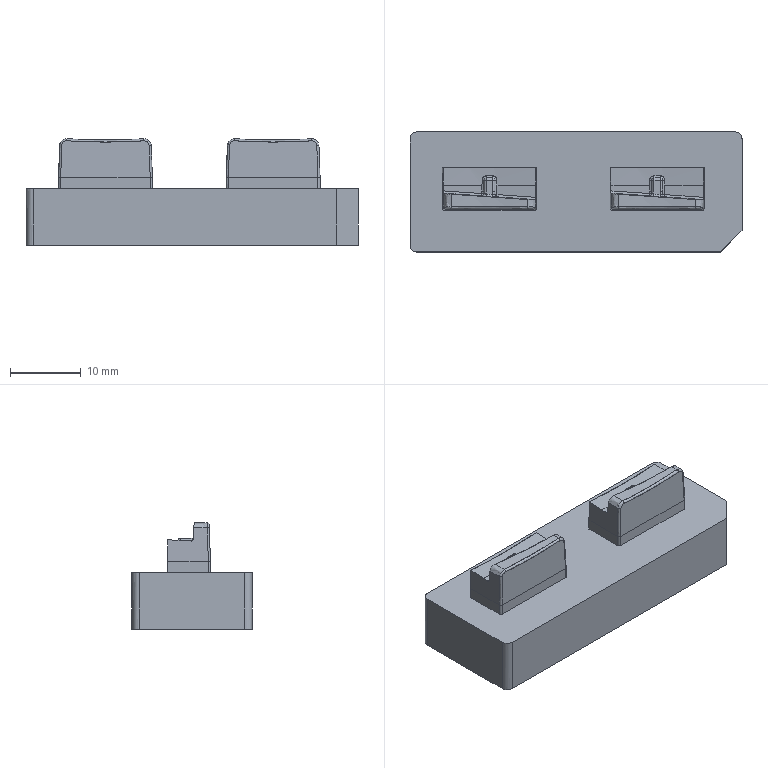NC program | PowerMill | posted with a generic post | part box 47 x 17 x 15.061 mm
Lines 1 to 1048 of 212044:
%
O0001
N104 ( POWERMILL CB  : 2026004.0)
N105 ( POST VER      : 2026.0.0.5161)
N106 ( OPTION FILE   : FANUC)
N107 ( OUTPUT WORKPLANE : WORLD)
N108 (  )
N109 ( TOOL LIST )
N110 (---------------------------------------)
N111 ( NO. | ID        | DIA.| TIP RAD|LENGTH)
N112 (---------------------------------------)
N113 (    1|D10C_1_1   |10.0 |  0.0   |70.52 )
N114 (    2|D4C_1_1    | 4.0 |  0.0   |62.24 )
N115 (   27|D1C_1_1    | 1.0 |  0.0   |58.04 )
N116 (    3|D10_1_1    |10.0 |  0.0   |70.24 )
N117 (    4|R1_1_1     | 2.0 |  1.0   |61.84 )
N118 (    6|R0.5_1_1   | 1.0 |  0.5   |58.16 )
N119 (   25|R0.3_1_1   | 0.6 |  0.3   |58.08 )
N120 (   13|TEXT_D4_1_1| 4.0 |  0.3   |62.32 )
N121 (---------------------------------------)
N122 (  )
N123 ( NUMBER OF TOOLPATHS: 13.0 )
N124 ( ESTIMATED PROGRAM DURATION: 0 HOURS 20 MIN 46 SEC)
N125 (  )
N126 G00 G21 G80 G40 G17
N127 G90
N128 G54
N129 G53 Z0.0
N130 (---------------)
N131 ( START TOOLPATH : 精公开粗01-扫面平行-D10C )
N132 (---------------)
N133 ( TOOL NO.    :1 )
N134 ( TOOL TYPE   : ENDMILL)
N135 ( TOOL ID     : D10C_1_1)
N136 ( TOOL DIA    : 10.0 LENGTH 70.52)
N137 T1
N138 M6
N139 S8000 M03
N140 G00 G90 X0.0 Y0.0
N141 G43 Z10.2 H1
N142
N143 G05 P10000 R4
N144 X31.28 Y11.28
N145 Z1.131
N146 G01 Z-0.069 F6000.0
N147 X26.28 F10000.0
N148 X-26.28
N149 Y5.64
N150 X26.28
N151 Y0.0
N152 X-26.28
N153 Y-5.64
N154 X26.28
N155 Y-11.28
N156 X-26.28
N157 X-31.28
N158 G00 Z10.2
N159 G05 P0
N160 (---------------)
N161 ( END TOOLPATH : 精公开粗01-扫面平行-D10C )
N162 (---------------)
N163 ( START TOOLPATH : 精公开粗01-外形偏置-D10C )
N164 (---------------)
N165 G00 X-0.2 Y0.0 Z9.881
N166 G05 P10000 R4
N167 X31.555 Y4.0124
N168 Z0.7186
N169 G01 Z-0.4814 F6000.0
N170 X31.0275 F10000.0
N171 G03 X26.28 Y-0.7351 I0.0 J-4.7475
N172 G01 Y-10.28
N173 G02 X25.28 Y-11.28 I-1.0 J0.0
N174 G01 X-25.68
N175 G02 X-26.68 Y-10.28 I0.0 J1.0
N176 G01 Y10.28
N177 G02 X-25.68 Y11.28 I1.0 J0.0
N178 G01 X25.28
N179 G02 X26.28 Y10.28 I0.0 J-1.0
N180 G01 Y-0.7351
N181 X22.9506 Y-0.9668
N182 X22.9641 Y-1.1601
N183 X22.933 Y-2.707
N184 X22.7913 Y-3.4804
N185 X22.5391 Y-4.2538
N186 X22.1429 Y-5.0273
N187 X21.5582 Y-5.8007
N188 X20.7183 Y-6.5741
N189 X19.9091 Y-7.0696
N190 X19.2573 Y-7.3476
N191 X18.3622 Y-7.5959
N192 X17.5888 Y-7.6917
N193 X16.8154 Y-7.7121
N194 X11.4014 Y-7.6611
N195 X11.3967
N196 X5.9874 Y-7.7126
N197 X5.214 Y-7.6816
N198 X4.4406 Y-7.5712
N199 X3.6738 Y-7.3476
N200 X2.8937 Y-7.0001
N201 X2.223 Y-6.5741
N202 X1.3803 Y-5.8007
N203 X0.7978 Y-5.0273
N204 X0.5734 Y-4.6294
N205 X0.4007 Y-4.2538
N206 X0.1489 Y-3.4804
N207 X0.0079 Y-2.707
N208 X-0.0194 Y-1.9336
N209 X-0.0237 Y-1.1757
N210 X-0.7788 Y-1.1601
N211 X-0.8107 Y-2.707
N212 X-0.9518 Y-3.4804
N213 X-1.2049 Y-4.2538
N214 X-1.6016 Y-5.0273
N215 X-1.7469 Y-5.2497
N216 X-2.1858 Y-5.8007
N217 X-2.5203 Y-6.1467
N218 X-3.0233 Y-6.5741
N219 X-3.2937 Y-6.7631
N220 X-4.0671 Y-7.1796
N221 X-4.4858 Y-7.3476
N222 X-4.8406 Y-7.4671
N223 X-5.614 Y-7.6365
N224 X-6.3874 Y-7.704
N225 X-11.8014 Y-7.6651
N226 X-11.805
N227 X-17.9888 Y-7.7098
N228 X-18.7622 Y-7.6593
N229 X-19.5357 Y-7.5155
N230 X-20.3091 Y-7.2523
N231 X-21.0825 Y-6.8685
N232 X-21.5226 Y-6.5741
N233 X-21.8559 Y-6.3049
N234 X-22.364 Y-5.8007
N235 X-22.6294 Y-5.4834
N236 X-22.9463 Y-5.0273
N237 X-23.3432 Y-4.2538
N238 X-23.594 Y-3.4804
N239 X-23.7368 Y-2.707
N240 X-23.7641 Y-1.9336
N241 X-23.7721 Y-0.3867
N242 X-23.73 Y0.3867
N243 X-23.573 Y1.1601
N244 X-23.4028 Y1.6681
N245 X-23.2893 Y1.9336
N246 X-22.8515 Y2.707
N247 X-22.6294 Y3.006
N248 X-22.2028 Y3.4804
N249 X-21.8559 Y3.795
N250 X-21.2044 Y4.2538
N251 X-20.3091 Y4.6806
N252 X-19.5357 Y4.8996
N253 X-18.7622 Y4.9981
N254 X-17.9888 Y4.9861
N255 X-5.614 Y4.1201
N256 X-4.8406 Y3.9942
N257 X-4.0671 Y3.7451
N258 X-3.2937 Y3.3525
N259 X-2.5203 Y2.773
N260 X-1.769 Y1.9336
N261 X-1.3083 Y1.1601
N262 X-1.005 Y0.3867
N263 X-0.8337 Y-0.3867
N264 X-0.7788 Y-1.1601
N265 X-0.0237 Y-1.1757
N266 X-0.0283 Y-0.3867
N267 X0.0143 Y0.3867
N268 X0.1704 Y1.1601
N269 X0.4548 Y1.9336
N270 X0.5734 Y2.177
N271 X0.8933 Y2.707
N272 X1.3469 Y3.2768
N273 X1.5396 Y3.4804
N274 X2.1203 Y3.9724
N275 X2.5408 Y4.2538
N276 X2.8937 Y4.4455
N277 X3.6671 Y4.7591
N278 X4.4406 Y4.9414
N279 X5.214 Y5.0062
N280 X5.9874 Y4.9703
N281 X17.5888 Y4.1592
N282 X18.3622 Y4.0955
N283 X19.1357 Y3.9326
N284 X19.9091 Y3.6434
N285 X20.2305 Y3.4804
N286 X20.6825 Y3.2017
N287 X21.2965 Y2.707
N288 X21.4559 Y2.5509
N289 X21.9755 Y1.9336
N290 X22.2294 Y1.5464
N291 X22.436 Y1.1601
N292 X22.7398 Y0.3867
N293 X22.9102 Y-0.3867
N294 X22.9506 Y-0.9668
N295 X26.28 Y-0.7351
N296 G00 Z3.3563
N297 G01 X31.555 Y4.0124
N298 G00 Z0.3563
N299 G01 Z-0.8437 F6000.0
N300 X31.0275 F10000.0
N301 G03 X26.28 Y-0.7351 I0.0 J-4.7475
N302 G01 Y-10.28
N303 G02 X25.28 Y-11.28 I-1.0 J0.0
N304 G01 X-25.68
N305 G02 X-26.68 Y-10.28 I0.0 J1.0
N306 G01 Y10.28
N307 G02 X-25.68 Y11.28 I1.0 J0.0
N308 G01 X25.28
N309 G02 X26.28 Y10.28 I0.0 J-1.0
N310 G01 Y-0.6564
N311 X23.1598 Y-0.8701
N312 X23.1797 Y-1.1601
N313 X23.1499 Y-2.707
N314 X23.0133 Y-3.4804
N315 X22.7652 Y-4.2538
N316 X22.3726 Y-5.0273
N317 X21.8112 Y-5.8007
N318 X21.4559 Y-6.1752
N319 X20.9868 Y-6.5741
N320 X20.6825 Y-6.7872
N321 X19.9091 Y-7.2199
N322 X19.6073 Y-7.3476
N323 X19.1357 Y-7.5058
N324 X18.3622 Y-7.6665
N325 X17.5888 Y-7.7263
N326 X5.214 Y-7.7236
N327 X4.4406 Y-7.6464
N328 X3.6671 Y-7.4647
N329 X3.33 Y-7.3476
N330 X2.8937 Y-7.1538
N331 X2.1203 Y-6.6982
N332 X1.9499 Y-6.5741
N333 X1.3469 Y-6.0418
N334 X1.1262 Y-5.8007
N335 X0.5734 Y-5.0459
N336 X0.1714 Y-4.2538
N337 X-0.0785 Y-3.4804
N338 X-0.2 Y-2.8258
N339 X-0.2395 Y-1.9336
N340 X-0.2407 Y-1.1666
N341 X-0.5638 Y-1.1601
N342 X-0.5945 Y-2.707
N343 X-0.7306 Y-3.4804
N344 X-0.9734 Y-4.2399
N345 X-1.3713 Y-5.0273
N346 X-1.7469 Y-5.5717
N347 X-1.9327 Y-5.8007
N348 X-2.5203 Y-6.3844
N349 X-2.7572 Y-6.5741
N350 X-3.2937 Y-6.9312
N351 X-4.1359 Y-7.3476
N352 X-4.8406 Y-7.5644
N353 X-5.614 Y-7.6964
N354 X-6.3874 Y-7.7263
N355 X-17.9888
N356 X-18.7622 Y-7.712
N357 X-19.5357 Y-7.6034
N358 X-20.3091 Y-7.3868
N359 X-21.0825 Y-7.0321
N360 X-21.7943 Y-6.5741
N361 X-22.6177 Y-5.8007
N362 X-23.1815 Y-5.0273
N363 X-23.4028 Y-4.6283
N364 X-23.5726 Y-4.2538
N365 X-23.8216 Y-3.4804
N366 X-23.9579 Y-2.707
N367 X-23.9838 Y-1.9336
N368 X-23.9863 Y-0.3867
N369 X-23.9489 Y0.3867
N370 X-23.7967 Y1.1601
N371 X-23.5169 Y1.9336
N372 X-23.085 Y2.707
N373 X-22.6294 Y3.2897
N374 X-22.4489 Y3.4804
N375 X-21.8559 Y3.9933
N376 X-21.4711 Y4.2538
N377 X-21.0825 Y4.4704
N378 X-20.3091 Y4.7847
N379 X-19.5357 Y4.9702
N380 X-19.0108 Y5.0273
N381 X-18.3916
N382 X-5.614 Y4.1345
N383 X-4.8406 Y4.0403
N384 X-4.0671 Y3.8286
N385 X-3.2937 Y3.4779
N386 X-2.5203 Y2.9594
N387 X-2.2308 Y2.707
N388 X-1.7469 Y2.1869
N389 X-1.5526 Y1.9336
N390 X-1.0916 Y1.1601
N391 X-0.7898 Y0.3867
N392 X-0.6172 Y-0.3867
N393 X-0.5638 Y-1.1601
N394 X-0.2407 Y-1.1666
N395 X-0.2419 Y-0.3867
N396 X-0.2049 Y0.3867
N397 X-0.0528 Y1.1601
N398 X0.227 Y1.9336
N399 X0.6588 Y2.707
N400 X1.295 Y3.4804
N401 X2.1203 Y4.1564
N402 X2.8937 Y4.5806
N403 X3.6671 Y4.8532
N404 X4.4406 Y5.0002
N405 X4.733 Y5.0273
N406 X5.3521
N407 X18.3622 Y4.117
N408 X19.1357 Y3.9899
N409 X19.9091 Y3.7381
N410 X20.4493 Y3.4804
N411 X20.6825 Y3.3428
N412 X21.4559 Y2.7598
N413 X22.1912 Y1.9336
N414 X22.6517 Y1.1601
N415 X22.9538 Y0.3867
N416 X23.1267 Y-0.3867
N417 X23.1598 Y-0.8701
N418 X26.28 Y-0.6564
N419 Y-0.7351
N420 G00 Z2.9939
N421 G01 X31.555 Y4.0124
N422 G00 Z-0.0061
N423 G01 Z-1.2061 F6000.0
N424 X31.0275 F10000.0
N425 G03 X26.28 Y-0.7351 I0.0 J-4.7475
N426 G01 Y-10.28
N427 G02 X25.28 Y-11.28 I-1.0 J0.0
N428 G01 X-25.68
N429 G02 X-26.68 Y-10.28 I0.0 J1.0
N430 G01 Y10.28
N431 G02 X-25.68 Y11.28 I1.0 J0.0
N432 G01 X25.28
N433 G02 X26.28 Y10.28 I0.0 J-1.0
N434 G01 Y-0.6635
N435 X23.2292 Y-0.8701
N436 X23.2489 Y-1.1601
N437 X23.2498 Y-1.9336
N438 X23.22 Y-2.707
N439 X23.0864 Y-3.4804
N440 X23.0028 Y-3.7922
N441 X22.8382 Y-4.2538
N442 X22.4558 Y-5.0273
N443 X22.2294 Y-5.3724
N444 X21.8943 Y-5.8007
N445 X21.4559 Y-6.2554
N446 X21.0766 Y-6.5741
N447 X20.6825 Y-6.8542
N448 X19.7198 Y-7.3476
N449 X19.1357 Y-7.5362
N450 X18.3622 Y-7.6927
N451 X17.5888 Y-7.7389
N452 X5.214 Y-7.7377
N453 X4.4406 Y-7.6676
N454 X3.6671 Y-7.4911
N455 X3.2539 Y-7.3476
N456 X2.8937 Y-7.1899
N457 X2.1203 Y-6.7382
N458 X1.8988 Y-6.5741
N459 X1.3469 Y-6.0901
N460 X1.0801 Y-5.8007
N461 X0.5734 Y-5.1141
N462 X0.1353 Y-4.2538
N463 X-0.1106 Y-3.4804
N464 X-0.2456 Y-2.707
N465 X-0.2739 Y-1.9336
N466 X-0.275 Y-1.1598
N467 X-0.4953 Y-1.1601
N468 X-0.4941 Y-1.9336
N469 X-0.5239 Y-2.707
N470 X-0.6575 Y-3.4804
N471 X-0.9062 Y-4.2538
N472 X-1.2902 Y-5.0273
N473 X-1.7469 Y-5.6768
N474 X-2.5203 Y-6.4571
N475 X-3.2937 Y-6.9965
N476 X-4.0257 Y-7.3476
N477 X-4.8406 Y-7.5957
N478 X-5.614 Y-7.7181
N479 X-6.3874 Y-7.739
N480 X-17.9888
N481 X-18.7622 Y-7.729
N482 X-19.5357 Y-7.6238
N483 X-20.3091 Y-7.4152
N484 X-21.0825 Y-7.0723
N485 X-21.8449 Y-6.5741
N486 X-22.6294 Y-5.8404
N487 X-23.2239 Y-5.0273
N488 X-23.4028 Y-4.7049
N489 X-23.6082 Y-4.2538
N490 X-23.8545 Y-3.4804
N491 X-23.9895 Y-2.707
N492 X-24.0181 Y-1.9336
N493 X-24.0202 Y-0.3867
N494 X-23.9845 Y0.3867
N495 X-23.8346 Y1.1601
N496 X-23.5576 Y1.9336
N497 X-23.4028 Y2.2496
N498 X-23.1294 Y2.707
N499 X-22.4987 Y3.4804
N500 X-21.8559 Y4.0347
N501 X-21.5315 Y4.2538
N502 X-21.0825 Y4.504
N503 X-20.3091 Y4.8136
N504 X-19.5357 Y4.9916
N505 X-18.7622 Y5.052
N506 X-18.2055 Y5.0273
N507 X-5.614 Y4.1468
N508 X-4.8406 Y4.061
N509 X-4.0671 Y3.8601
N510 X-3.2937 Y3.5252
N511 X-2.5203 Y3.0238
N512 X-2.1524 Y2.707
N513 X-1.7469 Y2.2795
N514 X-1.4777 Y1.9336
N515 X-1.0196 Y1.1601
N516 X-0.7189 Y0.3867
N517 X-0.5475 Y-0.3867
N518 X-0.4953 Y-1.1601
N519 X-0.275 Y-1.1598
N520 X-0.2761 Y-0.3867
N521 X-0.2406 Y0.3867
N522 X-0.0907 Y1.1601
N523 X0.1863 Y1.9336
N524 X0.5734 Y2.6446
N525 X1.2452 Y3.4804
N526 X2.1203 Y4.1951
N527 X2.8937 Y4.612
N528 X3.6671 Y4.8799
N529 X4.4406 Y5.0217
N530 X5.214 Y5.0476
N531 X18.3622 Y4.1306
N532 X19.1357 Y4.0139
N533 X19.9091 Y3.775
N534 X20.5348 Y3.4804
N535 X21.4559 Y2.8316
N536 X21.5916 Y2.707
N537 X22.2294 Y1.9853
N538 X22.7243 Y1.1601
N539 X23.0028 Y0.4646
N540 X23.1965 Y-0.3867
N541 X23.2292 Y-0.8701
N542 X26.28 Y-0.6635
N543 Y-0.7351
N544 G00 Z2.6316
N545 G01 X31.555 Y4.0124
N546 G00 Z-0.3684
N547 G01 Z-1.5684 F6000.0
N548 X31.0275 F10000.0
N549 G03 X26.28 Y-0.7351 I0.0 J-4.7475
N550 G01 Y-10.28
N551 G02 X25.28 Y-11.28 I-1.0 J0.0
N552 G01 X-25.68
N553 G02 X-26.68 Y-10.28 I0.0 J1.0
N554 G01 Y10.28
N555 G02 X-25.68 Y11.28 I1.0 J0.0
N556 G01 X25.28
N557 G02 X26.28 Y10.28 I0.0 J-1.0
N558 G01 Y-0.6677
N559 X23.2442 Y-0.8701
N560 X23.2636 Y-1.1601
N561 X23.2497 Y-1.906
N562 X23.2498 Y-1.9336
N563 X23.2487 Y-1.9607
N564 X23.2349 Y-2.707
N565 X23.0975 Y-3.4804
N566 X23.0181 Y-3.7348
N567 X23.0027 Y-3.7922
N568 X22.9828 Y-3.8482
N569 X22.8562 Y-4.2538
N570 X22.4758 Y-5.0273
N571 X22.2294 Y-5.4027
N572 X21.9126 Y-5.8007
N573 X21.4559 Y-6.2702
N574 X21.1046 Y-6.5741
N575 X20.6825 Y-6.8757
N576 X19.7593 Y-7.3476
N577 X19.1357 Y-7.5492
N578 X18.3622 Y-7.7072
N579 X17.5888 Y-7.7516
N580 X5.214 Y-7.7508
N581 X4.4406 Y-7.6821
N582 X3.6671 Y-7.5068
N583 X3.2105 Y-7.3476
N584 X2.8937 Y-7.2084
N585 X2.1203 Y-6.7594
N586 X1.8704 Y-6.5741
N587 X1.3469 Y-6.1142
N588 X1.0572 Y-5.8007
N589 X0.5734 Y-5.1464
N590 X0.118 Y-4.2538
N591 X-0.1259 Y-3.4804
N592 X-0.2595 Y-2.707
N593 X-0.2868 Y-1.9336
N594 X-0.2879 Y-1.1637
N595 X-0.4804 Y-1.1601
N596 X-0.4942 Y-1.9081
N597 Y-1.9336
N598 X-0.4952 Y-1.9592
N599 X-0.509 Y-2.707
N600 X-0.6465 Y-3.4804
N601 X-0.8878 Y-4.2538
N602 X-1.2681 Y-5.0273
N603 X-1.7469 Y-5.7022
N604 X-2.5203 Y-6.4773
N605 X-3.2937 Y-7.0165
N606 X-3.9846 Y-7.3476
N607 X-4.8406 Y-7.6084
N608 X-5.614 Y-7.7317
N609 X-6.3874 Y-7.7516
N610 X-17.9888
N611 X-18.7622 Y-7.7422
N612 X-19.5357 Y-7.6389
N613 X-20.3091 Y-7.4317
N614 X-21.0825 Y-7.0914
N615 X-21.8559 Y-6.5876
N616 X-22.6294 Y-5.8665
N617 X-23.244 Y-5.0273
N618 X-23.4028 Y-4.7419
N619 X-23.6245 Y-4.2538
N620 X-23.8698 Y-3.4804
N621 X-24.0032 Y-2.707
N622 X-24.0307 Y-1.9336
N623 X-24.0329 Y-0.3867
N624 X-23.9988 Y0.3867
N625 X-23.851 Y1.1601
N626 X-23.5763 Y1.9336
N627 X-23.4028 Y2.2866
N628 X-23.1511 Y2.707
N629 X-22.6294 Y3.3704
N630 X-21.8559 Y4.0574
N631 X-21.5657 Y4.2538
N632 X-21.0825 Y4.5239
N633 X-20.3091 Y4.8313
N634 X-19.5357 Y5.0071
N635 X-18.7622 Y5.066
N636 X-17.9888 Y5.0248
N637 X-5.614 Y4.1595
N638 X-4.8406 Y4.0757
N639 X-4.0671 Y3.8767
N640 X-3.2937 Y3.5454
N641 X-2.5203 Y3.0461
N642 X-2.126 Y2.707
N643 X-1.7469 Y2.3076
N644 X-1.4551 Y1.9336
N645 X-0.9995 Y1.1601
N646 X-0.7008 Y0.3867
N647 X-0.5319 Y-0.3867
N648 X-0.4804 Y-1.1601
N649 X-0.2879 Y-1.1637
N650 X-0.289 Y-0.3867
N651 X-0.255 Y0.3867
N652 X-0.107 Y1.1601
N653 X0.1676 Y1.9336
N654 X0.5734 Y2.6776
N655 X1.2193 Y3.4804
N656 X1.3469 Y3.6063
N657 X2.1203 Y4.2169
N658 X2.8937 Y4.631
N659 X3.6671 Y4.8967
N660 X4.3576 Y5.0273
N661 X5.214 Y5.0606
N662 X18.3622 Y4.1432
N663 X19.1357 Y4.0299
N664 X19.9091 Y3.7932
N665 X20.569 Y3.4804
N666 X21.4559 Y2.8547
N667 X21.6179 Y2.707
N668 X22.2294 Y2.0157
N669 X22.7444 Y1.1601
N670 X23.0028 Y0.5146
N671 X23.212 Y-0.3867
N672 X23.2442 Y-0.8701
N673 X26.28 Y-0.6677
N674 Y-0.7351
N675 G00 Z2.2692
N676 G01 X31.555 Y4.0124
N677 G00 Z-0.7308
N678 G01 Z-1.9308 F6000.0
N679 X31.0275 F10000.0
N680 G03 X26.28 Y-0.7351 I0.0 J-4.7475
N681 G01 Y-10.28
N682 G02 X25.28 Y-11.28 I-1.0 J0.0
N683 G01 X-25.68
N684 G02 X-26.68 Y-10.28 I0.0 J1.0
N685 G01 Y10.28
N686 G02 X-25.68 Y11.28 I1.0 J0.0
N687 G01 X25.28
N688 G02 X26.28 Y10.28 I0.0 J-1.0
N689 G01 Y-0.675
N690 X23.2575 Y-0.8701
N691 X23.2762 Y-1.1601
N692 X23.2487 Y-2.707
N693 X23.1133 Y-3.4804
N694 X22.8738 Y-4.2538
N695 X22.4958 Y-5.0273
N696 X22.2294 Y-5.4327
N697 X21.936 Y-5.8007
N698 X21.4559 Y-6.2944
N699 X21.1329 Y-6.5741
N700 X20.6825 Y-6.8962
N701 X19.8034 Y-7.3476
N702 X19.1357 Y-7.5652
N703 X18.3622 Y-7.7216
N704 X17.5888 Y-7.7643
N705 X5.214 Y-7.7639
N706 X4.4406 Y-7.6967
N707 X3.6671 Y-7.5225
N708 X3.1671 Y-7.3476
N709 X2.8937 Y-7.227
N710 X2.1203 Y-6.7806
N711 X1.842 Y-6.5741
N712 X1.3469 Y-6.1377
N713 X1.0343 Y-5.8007
N714 X0.5734 Y-5.1788
N715 X0.1007 Y-4.2538
N716 X-0.1413 Y-3.4804
N717 X-0.2734 Y-2.707
N718 X-0.2994 Y-1.9336
N719 X-0.3005 Y-1.1631
N720 X-0.4677 Y-1.1601
N721 X-0.4952 Y-2.707
N722 X-0.6307 Y-3.4804
N723 X-0.8703 Y-4.2538
N724 X-0.9734 Y-4.4996
N725 X-1.2481 Y-5.0273
N726 X-1.7469 Y-5.7298
N727 X-2.5203 Y-6.5005
N728 X-3.2937 Y-7.0362
N729 X-3.9405 Y-7.3476
N730 X-4.8406 Y-7.6239
N731 X-5.614 Y-7.7454
N732 X-6.3874 Y-7.7643
N733 X-17.9888
N734 X-18.7622 Y-7.7555
N735 X-19.5357 Y-7.654
N736 X-20.3091 Y-7.4482
N737 X-20.5775 Y-7.3476
N738 X-21.0825 Y-7.1106
N739 X-21.8559 Y-6.6098
N740 X-22.6294 Y-5.8926
N741 X-23.264 Y-5.0273
N742 X-23.4028 Y-4.779
N743 X-23.642 Y-4.2538
N744 X-23.8852 Y-3.4804
N745 X-24.017 Y-2.707
N746 X-24.0434 Y-1.9336
N747 X-24.0455 Y-0.3867
N748 X-24.013 Y0.3867
N749 X-23.8673 Y1.1601
N750 X-23.595 Y1.9336
N751 X-23.4028 Y2.3236
N752 X-23.1727 Y2.707
N753 X-22.6294 Y3.3976
N754 X-21.8559 Y4.0802
N755 X-21.5998 Y4.2538
N756 X-21.0825 Y4.5437
N757 X-20.3091 Y4.8491
N758 X-19.5357 Y5.0225
N759 X-18.7622 Y5.08
N760 X-17.9888 Y5.0377
N761 X-5.614 Y4.1722
N762 X-4.8406 Y4.0904
N763 X-4.0671 Y3.8933
N764 X-3.2937 Y3.5643
N765 X-2.5203 Y3.068
N766 X-2.101 Y2.707
N767 X-1.7469 Y2.3342
N768 X-1.4341 Y1.9336
N769 X-0.9812 Y1.1601
N770 X-0.6847 Y0.3867
N771 X-0.5176 Y-0.3867
N772 X-0.4677 Y-1.1601
N773 X-0.3005 Y-1.1631
N774 X-0.3016 Y-0.3867
N775 X-0.2694 Y0.3867
N776 X-0.1234 Y1.1601
N777 X0.1489 Y1.9336
N778 X0.5711 Y2.707
N779 X1.1934 Y3.4804
N780 X1.3469 Y3.6319
N781 X2.1203 Y4.2387
N782 X2.8937 Y4.6501
N783 X3.6671 Y4.9136
N784 X4.2419 Y5.0273
N785 X5.214 Y5.0737
N786 X18.3622 Y4.1559
N787 X19.1357 Y4.0449
N788 X19.9091 Y3.81
N789 X20.6026 Y3.4804
N790 X21.4559 Y2.8778
N791 X21.643 Y2.707
N792 X22.2294 Y2.0447
N793 X22.7627 Y1.1601
N794 X23.0028 Y0.5646
N795 X23.2263 Y-0.3867
N796 X23.2575 Y-0.8701
N797 X26.28 Y-0.675
N798 Y-0.7351
N799 G00 Z1.9069
N800 G01 X31.555 Y4.0124
N801 G00 Z-1.0931
N802 G01 Z-2.2931 F6000.0
N803 X31.0275 F10000.0
N804 G03 X26.28 Y-0.7351 I0.0 J-4.7475
N805 G01 Y-0.7793
N806 X23.2768 Y-0.9668
N807 X23.2889 Y-1.1601
N808 X23.2624 Y-2.707
N809 X23.1291 Y-3.4804
N810 X22.8913 Y-4.2538
N811 X22.5157 Y-5.0273
N812 X22.2294 Y-5.4628
N813 X21.9593 Y-5.8007
N814 X21.4559 Y-6.3186
N815 X21.1611 Y-6.5741
N816 X20.6825 Y-6.9167
N817 X19.8475 Y-7.3476
N818 X19.1357 Y-7.5811
N819 X18.3622 Y-7.736
N820 X17.5888 Y-7.7769
N821 X5.214 Y-7.7766
N822 X4.4406 Y-7.7112
N823 X3.6671 Y-7.5382
N824 X2.8937 Y-7.2455
N825 X2.1203 Y-6.8019
N826 X1.8137 Y-6.5741
N827 X1.3469 Y-6.1612
N828 X1.0115 Y-5.8007
N829 X0.4601 Y-5.0273
N830 X0.0834 Y-4.2538
N831 X-0.1566 Y-3.4804
N832 X-0.2871 Y-2.707
N833 X-0.3121 Y-1.9336
N834 X-0.3132 Y-1.1626
N835 X-0.4551 Y-1.1601
N836 X-0.4814 Y-2.707
N837 X-0.615 Y-3.4804
N838 X-0.8529 Y-4.2538
N839 X-0.9734 Y-4.5402
N840 X-1.2282 Y-5.0273
N841 X-1.7469 Y-5.7575
N842 X-2.5203 Y-6.5236
N843 X-3.2937 Y-7.0558
N844 X-3.8963 Y-7.3476
N845 X-4.8406 Y-7.6394
N846 X-5.614 Y-7.759
N847 X-6.3874 Y-7.7769
N848 X-17.9888
N849 X-18.7622 Y-7.7687
N850 X-19.5357 Y-7.6692
N851 X-20.3091 Y-7.4647
N852 X-20.6206 Y-7.3476
N853 X-21.0825 Y-7.1298
N854 X-21.8559 Y-6.632
N855 X-22.6294 Y-5.9187
N856 X-23.2841 Y-5.0273
N857 X-23.6594 Y-4.2538
N858 X-23.9005 Y-3.4804
N859 X-24.0307 Y-2.707
N860 X-24.056 Y-1.9336
N861 X-24.0582 Y-0.3867
N862 X-24.0273 Y0.3867
N863 X-23.8836 Y1.1601
N864 X-23.6137 Y1.9336
N865 X-23.4028 Y2.3606
N866 X-23.1944 Y2.707
N867 X-22.6294 Y3.4249
N868 X-21.8559 Y4.1029
N869 X-21.6339 Y4.2538
N870 X-21.0825 Y4.5636
N871 X-20.3091 Y4.8668
N872 X-19.6048 Y5.0273
N873 X-18.7622 Y5.094
N874 X-17.9888 Y5.0507
N875 X-13.4444 Y4.7324
N876 X-12.5748 Y4.7831
N877 X-11.028 Y4.6615
N878 X-10.2545 Y4.5094
N879 X-10.2235 Y4.5072
N880 X-5.614 Y4.1849
N881 X-4.8406 Y4.1051
N882 X-4.0671 Y3.9099
N883 X-3.2937 Y3.5832
N884 X-2.5203 Y3.0899
N885 X-2.0759 Y2.707
N886 X-1.7469 Y2.3608
N887 X-1.4131 Y1.9336
N888 X-0.9734 Y1.1822
N889 X-0.6685 Y0.3867
N890 X-0.5033 Y-0.3867
N891 X-0.4551 Y-1.1601
N892 X-0.3132 Y-1.1626
N893 X-0.3143 Y-0.3867
N894 X-0.2838 Y0.3867
N895 X-0.1398 Y1.1601
N896 X0.1302 Y1.9336
N897 X0.5494 Y2.707
N898 X1.1674 Y3.4804
N899 X1.3469 Y3.6575
N900 X2.1099 Y4.2538
N901 X2.8937 Y4.6691
N902 X3.6671 Y4.9304
N903 X4.4406 Y5.0664
N904 X5.214 Y5.0867
N905 X9.8545 Y4.7636
N906 X11.4014 Y4.7675
N907 X12.1748 Y4.7133
N908 X12.9482 Y4.6205
N909 X13.7217 Y4.4931
N910 X13.745 Y4.4915
N911 X18.3622 Y4.1686
N912 X19.1357 Y4.06
N913 X19.9091 Y3.8267
N914 X20.6361 Y3.4804
N915 X21.4559 Y2.9009
N916 X21.668 Y2.707
N917 X22.2294 Y2.0737
N918 X22.781 Y1.1601
N919 X23.0764 Y0.3867
N920 X23.2406 Y-0.3867
N921 X23.2768 Y-0.9668
N922 X26.28 Y-0.7793
N923 Y-10.28
N924 G02 X25.28 Y-11.28 I-1.0 J0.0
N925 G01 X-25.68
N926 G02 X-26.68 Y-10.28 I0.0 J1.0
N927 G01 Y10.28
N928 G02 X-25.68 Y11.28 I1.0 J0.0
N929 G01 X25.28
N930 G02 X26.28 Y10.28 I0.0 J-1.0
N931 G01 Y-0.7351
N932 G00 Z1.5088
N933 G01 X31.555 Y4.0124
N934 G00 Z-1.4912
N935 G01 Z-2.6912 F6000.0
N936 X31.0275 F10000.0
N937 G03 X26.28 Y-0.7351 I0.0 J-4.7475
N938 G01 Y-10.28
N939 G02 X25.28 Y-11.28 I-1.0 J0.0
N940 G01 X-25.68
N941 G02 X-26.68 Y-10.28 I0.0 J1.0
N942 G01 Y10.28
N943 G02 X-25.68 Y11.28 I1.0 J0.0
N944 G01 X5.2182
N945 X5.214 Y8.736
N946 X6.7608 Y8.7335
N947 X8.3077 Y8.664
N948 X9.0811 Y8.5546
N949 X9.8545 Y8.3219
N950 X10.3635 Y8.121
N951 X11.1399 Y7.5862
N952 G03 X11.6756 Y7.5662 I0.2836 J0.4118
N953 G01 X12.626 Y8.121
N954 X12.9482 Y8.2565
N955 X13.7217 Y8.516
N956 X14.4951 Y8.6486
N957 X16.042 Y8.7312
N958 X18.3622 Y8.7218
N959 X19.1357 Y8.6166
N960 X19.9091 Y8.386
N961 X20.5018 Y8.121
N962 X20.6825 Y8.0172
N963 X21.4559 Y7.4713
N964 X21.5967 Y7.3476
N965 X22.2294 Y6.6541
N966 X22.76 Y5.8007
N967 X23.0028 Y5.2285
N968 X23.2483 Y4.2538
N969 X23.3092 Y3.4804
N970 X23.2699 Y-0.3867
N971 X23.3028 Y-1.1601
N972 X23.2775 Y-2.707
N973 X23.1465 Y-3.4804
N974 X22.9105 Y-4.2538
N975 X22.5376 Y-5.0273
N976 X22.2294 Y-5.4957
N977 X21.985 Y-5.8007
N978 X21.4559 Y-6.3452
N979 X21.1922 Y-6.5741
N980 X20.6825 Y-6.9392
N981 X19.8959 Y-7.3476
N982 X19.1357 Y-7.5986
N983 X18.3622 Y-7.7518
N984 X17.5888 Y-7.7908
N985 X5.214 Y-7.7905
N986 X4.4406 Y-7.7272
N987 X3.6671 Y-7.5555
N988 X2.8937 Y-7.2658
N989 X2.1203 Y-6.8252
N990 X1.7828 Y-6.5741
N991 X1.3469 Y-6.1871
N992 X0.9864 Y-5.8007
N993 X0.5734 Y-5.2466
N994 X0.4382 Y-5.0273
N995 X0.0644 Y-4.2538
N996 X-0.1734 Y-3.4804
N997 X-0.3022 Y-2.707
N998 X-0.326 Y-1.9336
N999 X-0.3329 Y3.4794
N1000 X-0.4368 Y3.4804
N1001 X-0.4739 Y-0.3867
N1002 X-0.4412 Y-1.1601
N1003 X-0.4662 Y-2.707
N1004 X-0.5977 Y-3.4804
N1005 X-0.8337 Y-4.2538
N1006 X-0.9734 Y-4.5835
N1007 X-1.2062 Y-5.0273
N1008 X-1.7469 Y-5.7878
N1009 X-2.5203 Y-6.5491
N1010 X-3.2937 Y-7.0774
N1011 X-3.8478 Y-7.3476
N1012 X-4.0671 Y-7.4326
N1013 X-4.8406 Y-7.6564
N1014 X-5.614 Y-7.774
N1015 X-6.3874 Y-7.7909
N1016 X-17.9888
N1017 X-18.7622 Y-7.7833
N1018 X-19.5357 Y-7.6858
N1019 X-20.3091 Y-7.4828
N1020 X-20.6667 Y-7.3476
N1021 X-21.0825 Y-7.1509
N1022 X-21.8559 Y-6.6565
N1023 X-22.6294 Y-5.9474
N1024 X-22.7578 Y-5.8007
N1025 X-23.3061 Y-5.0273
N1026 X-23.6785 Y-4.2538
N1027 X-23.9173 Y-3.4804
N1028 X-24.0458 Y-2.707
N1029 X-24.0699 Y-1.9336
N1030 X-24.0557 Y0.3867
N1031 X-24.0761 Y3.4804
N1032 X-24.0154 Y4.2538
N1033 X-23.8362 Y5.0273
N1034 X-23.5256 Y5.8007
N1035 X-23.4028 Y6.0377
N1036 X-23.0563 Y6.5741
N1037 X-22.6294 Y7.0865
N1038 X-22.3637 Y7.3476
N1039 X-21.8559 Y7.7594
N1040 X-21.2683 Y8.121
N1041 X-20.3091 Y8.5113
N1042 X-19.5357 Y8.6838
N1043 X-18.7622 Y8.736
N1044 X-17.2154 Y8.7359
N1045 X-15.6685 Y8.6824
N1046 X-14.8951 Y8.6008
N1047 X-14.1217 Y8.4245
N1048 X-13.3483 Y8.1006
N1049 X-12.6737 Y7.6727
N1050 X-12.611 Y7.6389
N1051 X-12.5441 Y7.6144
N1052 G03 X-11.9672 Y7.5938 I0.303 J0.3977
N1053 G01 X-11.118 Y8.121
N1054 X-10.2545 Y8.4459
N1055 X-9.4811 Y8.6129
N1056 X-7.9343 Y8.7254
N1057 X-5.614 Y8.735
N1058 X-4.8406 Y8.6606
N1059 X-4.0671 Y8.4671
N1060 X-3.2937 Y8.1464
N1061 X-2.5203 Y7.658
N1062 X-2.1486 Y7.3476
N1063 X-1.7469 Y6.9371
N1064 X-1.4548 Y6.5741
N1065 X-0.9839 Y5.8007
N1066 X-0.6772 Y5.0273
N1067 X-0.4959 Y4.2538
N1068 X-0.4368 Y3.4804
N1069 X-0.3329 Y3.4794
N1070 Y3.4804
N1071 X-0.2729 Y4.2538
N1072 X-0.0943 Y5.0273
N1073 X0.2165 Y5.8007
N1074 X0.6876 Y6.5741
N1075 X1.3469 Y7.3188
N1076 X2.1203 Y7.9134
N1077 X2.4756 Y8.121
N1078 X2.8937 Y8.316
N1079 X3.6671 Y8.5741
N1080 X4.4406 Y8.7083
N1081 X5.214 Y8.736
N1082 X5.2182 Y11.28
N1083 X25.28
N1084 G02 X26.28 Y10.28 I0.0 J-1.0
N1085 G01 Y-0.7351
N1086 G00 Z1.1107
N1087 G01 X31.555 Y4.0124
N1088 G00 Z-1.8893
N1089 G01 Z-3.0893 F6000.0
N1090 X31.0275 F10000.0
N1091 G03 X26.28 Y-0.7351 I0.0 J-4.7475
N1092 G01 Y-10.28
N1093 G02 X25.28 Y-11.28 I-1.0 J0.0
N1094 G01 X-25.68
N1095 G02 X-26.68 Y-10.28 I0.0 J1.0
N1096 G01 Y10.28
N1097 G02 X-25.68 Y11.28 I1.0 J0.0
N1098 G01 X4.3642
N1099 X4.4406 Y8.713
N1100 X5.214 Y8.736
N1101 X17.5888
N1102 X18.3622 Y8.7248
N1103 X19.1357 Y8.6217
N1104 X19.9091 Y8.3952
N1105 X20.2609 Y8.2286
N1106 X20.5018 Y8.1209
N1107 X20.5652 Y8.0845
N1108 X20.6825 Y8.029
N1109 X21.4559 Y7.4847
N1110 X21.6116 Y7.3476
N1111 X22.2294 Y6.6733
N1112 X22.774 Y5.8007
N1113 X23.0839 Y5.0273
N1114 X23.2625 Y4.2538
N1115 X23.3231 Y3.4804
N1116 X23.3156 Y-1.9336
N1117 X23.2926 Y-2.707
N1118 X23.1639 Y-3.4804
N1119 X22.9297 Y-4.2538
N1120 X22.5596 Y-5.0273
N1121 X22.2294 Y-5.5277
N1122 X22.0107 Y-5.8007
N1123 X21.4559 Y-6.3718
N1124 X21.2232 Y-6.5741
N1125 X20.6825 Y-6.9617
N1126 X19.9425 Y-7.3476
N1127 X19.1357 Y-7.6162
N1128 X18.3622 Y-7.7673
N1129 X17.5888 Y-7.8047
N1130 X5.214 Y-7.8045
N1131 X4.4406 Y-7.7432
N1132 X3.6671 Y-7.5728
N1133 X3.031 Y-7.3476
N1134 X2.1203 Y-6.8485
N1135 X1.7522 Y-6.5741
N1136 X1.3469 Y-6.2129
N1137 X0.9613 Y-5.8007
N1138 X0.5734 Y-5.2821
N1139 X0.4162 Y-5.0273
N1140 X0.0454 Y-4.2538
N1141 X-0.1903 Y-3.4804
N1142 X-0.3173 Y-2.707
N1143 X-0.3399 Y-1.9336
N1144 X-0.3474 Y3.4803
N1145 X-0.4209 Y3.4804